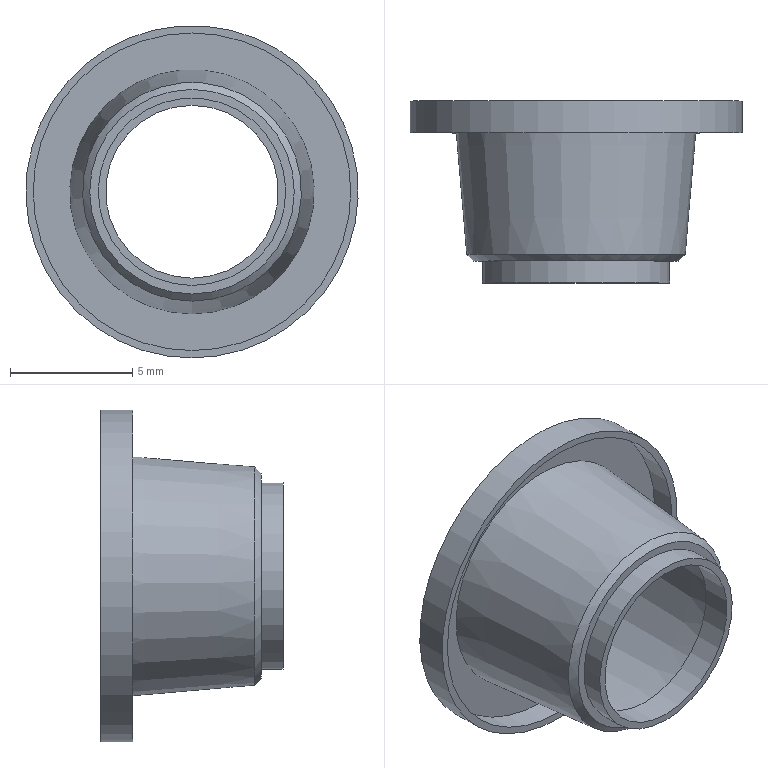Part | NX | features DATUM_CSYS 3, SKETCH 2, SWP104 1 | 1 solid | 13 faces | box 13.6 x 7.451 x 13.6 mm | volume 99.127 mm3 | plane 6 | cylinder 4 | cone 3 | commonest cylinder face diameters 7.073 x1 7.673 x1 13 x1 13.6 x1
STEP:
#1=CARTESIAN_POINT('',(0.,0.,-5.));
#2=VERTEX_POINT('',#1);
#3=CARTESIAN_POINT('',(0.,0.,0.));
#4=DIRECTION('',(0.,-1.,0.));
#5=DIRECTION('',(0.,0.,-1.));
#6=AXIS2_PLACEMENT_3D('',#3,#4,#5);
#7=CIRCLE('',#6,5.);
#8=EDGE_CURVE('',#2,#2,#7,.T.);
#9=ORIENTED_EDGE('',*,*,#8,.T.);
#10=EDGE_LOOP('',(#9));
#11=FACE_BOUND('',#10,.T.);
#12=CARTESIAN_POINT('',(0.,-5.977,-4.477));
#13=VERTEX_POINT('',#12);
#14=CARTESIAN_POINT('',(0.,-5.977,0.));
#15=DIRECTION('',(0.,-1.,0.));
#16=DIRECTION('',(0.,0.,-1.));
#17=AXIS2_PLACEMENT_3D('',#14,#15,#16);
#18=CIRCLE('',#17,4.477);
#19=EDGE_CURVE('',#13,#13,#18,.T.);
#20=ORIENTED_EDGE('',*,*,#19,.F.);
#21=EDGE_LOOP('',(#20));
#22=FACE_BOUND('',#21,.T.);
#23=CARTESIAN_POINT('',(0.,-5.977,0.));
#24=DIRECTION('',(0.,1.,0.));
#25=DIRECTION('',(0.,0.,1.));
#26=AXIS2_PLACEMENT_3D('',#23,#24,#25);
#27=CONICAL_SURFACE('',#26,4.477,0.08727);
#28=ADVANCED_FACE('',(#11,#22),#27,.T.);
#29=CARTESIAN_POINT('',(0.,0.,-6.5));
#30=VERTEX_POINT('',#29);
#31=CARTESIAN_POINT('',(0.,0.,0.));
#32=DIRECTION('',(0.,-1.,0.));
#33=DIRECTION('',(0.,0.,-1.));
#34=AXIS2_PLACEMENT_3D('',#31,#32,#33);
#35=CIRCLE('',#34,6.5);
#36=EDGE_CURVE('',#30,#30,#35,.T.);
#37=ORIENTED_EDGE('',*,*,#36,.T.);
#38=EDGE_LOOP('',(#37));
#39=FACE_BOUND('',#38,.T.);
#40=ORIENTED_EDGE('',*,*,#8,.F.);
#41=EDGE_LOOP('',(#40));
#42=FACE_BOUND('',#41,.T.);
#43=CARTESIAN_POINT('',(0.,0.,5.));
#44=DIRECTION('',(0.,-1.,0.));
#45=DIRECTION('',(0.,0.,-1.));
#46=AXIS2_PLACEMENT_3D('',#43,#44,#45);
#47=PLANE('',#46);
#48=ADVANCED_FACE('',(#39,#42),#47,.T.);
#49=CARTESIAN_POINT('',(0.,-1.,-6.5));
#50=VERTEX_POINT('',#49);
#51=CARTESIAN_POINT('',(0.,-1.,0.));
#52=DIRECTION('',(0.,-1.,0.));
#53=DIRECTION('',(0.,0.,-1.));
#54=AXIS2_PLACEMENT_3D('',#51,#52,#53);
#55=CIRCLE('',#54,6.5);
#56=EDGE_CURVE('',#50,#50,#55,.T.);
#57=ORIENTED_EDGE('',*,*,#56,.T.);
#58=EDGE_LOOP('',(#57));
#59=FACE_BOUND('',#58,.T.);
#60=ORIENTED_EDGE('',*,*,#36,.F.);
#61=EDGE_LOOP('',(#60));
#62=FACE_BOUND('',#61,.T.);
#63=CARTESIAN_POINT('',(0.,0.,0.));
#64=DIRECTION('',(0.,-1.,0.));
#65=DIRECTION('',(0.,0.,-1.));
#66=AXIS2_PLACEMENT_3D('',#63,#64,#65);
#67=CYLINDRICAL_SURFACE('',#66,6.5);
#68=ADVANCED_FACE('',(#59,#62),#67,.F.);
#69=CARTESIAN_POINT('',(0.,-1.,-6.8));
#70=VERTEX_POINT('',#69);
#71=CARTESIAN_POINT('',(0.,-1.,0.));
#72=DIRECTION('',(0.,-1.,0.));
#73=DIRECTION('',(0.,0.,-1.));
#74=AXIS2_PLACEMENT_3D('',#71,#72,#73);
#75=CIRCLE('',#74,6.8);
#76=EDGE_CURVE('',#70,#70,#75,.T.);
#77=ORIENTED_EDGE('',*,*,#76,.T.);
#78=EDGE_LOOP('',(#77));
#79=FACE_BOUND('',#78,.T.);
#80=ORIENTED_EDGE('',*,*,#56,.F.);
#81=EDGE_LOOP('',(#80));
#82=FACE_BOUND('',#81,.T.);
#83=CARTESIAN_POINT('',(0.,-1.,6.5));
#84=DIRECTION('',(0.,-1.,0.));
#85=DIRECTION('',(0.,0.,-1.));
#86=AXIS2_PLACEMENT_3D('',#83,#84,#85);
#87=PLANE('',#86);
#88=ADVANCED_FACE('',(#79,#82),#87,.T.);
#89=CARTESIAN_POINT('',(0.,0.3,-6.8));
#90=VERTEX_POINT('',#89);
#91=CARTESIAN_POINT('',(0.,0.3,0.));
#92=DIRECTION('',(0.,-1.,0.));
#93=DIRECTION('',(0.,0.,-1.));
#94=AXIS2_PLACEMENT_3D('',#91,#92,#93);
#95=CIRCLE('',#94,6.8);
#96=EDGE_CURVE('',#90,#90,#95,.T.);
#97=ORIENTED_EDGE('',*,*,#96,.T.);
#98=EDGE_LOOP('',(#97));
#99=FACE_BOUND('',#98,.T.);
#100=ORIENTED_EDGE('',*,*,#76,.F.);
#101=EDGE_LOOP('',(#100));
#102=FACE_BOUND('',#101,.T.);
#103=CARTESIAN_POINT('',(0.,0.,0.));
#104=DIRECTION('',(0.,-1.,0.));
#105=DIRECTION('',(0.,0.,-1.));
#106=AXIS2_PLACEMENT_3D('',#103,#104,#105);
#107=CYLINDRICAL_SURFACE('',#106,6.8);
#108=ADVANCED_FACE('',(#99,#102),#107,.T.);
#109=CARTESIAN_POINT('',(0.,0.3,-4.725));
#110=VERTEX_POINT('',#109);
#111=CARTESIAN_POINT('',(0.,0.3,0.));
#112=DIRECTION('',(0.,-1.,0.));
#113=DIRECTION('',(0.,0.,-1.));
#114=AXIS2_PLACEMENT_3D('',#111,#112,#113);
#115=CIRCLE('',#114,4.725);
#116=EDGE_CURVE('',#110,#110,#115,.T.);
#117=ORIENTED_EDGE('',*,*,#116,.T.);
#118=EDGE_LOOP('',(#117));
#119=FACE_BOUND('',#118,.T.);
#120=ORIENTED_EDGE('',*,*,#96,.F.);
#121=EDGE_LOOP('',(#120));
#122=FACE_BOUND('',#121,.T.);
#123=CARTESIAN_POINT('',(0.,0.3,6.8));
#124=DIRECTION('',(0.,1.,0.));
#125=DIRECTION('',(0.,0.,1.));
#126=AXIS2_PLACEMENT_3D('',#123,#124,#125);
#127=PLANE('',#126);
#128=ADVANCED_FACE('',(#119,#122),#127,.T.);
#129=CARTESIAN_POINT('',(0.,-5.951,-4.178));
#130=VERTEX_POINT('',#129);
#131=CARTESIAN_POINT('',(0.,-5.951,0.));
#132=DIRECTION('',(0.,-1.,0.));
#133=DIRECTION('',(0.,0.,-1.));
#134=AXIS2_PLACEMENT_3D('',#131,#132,#133);
#135=CIRCLE('',#134,4.178);
#136=EDGE_CURVE('',#130,#130,#135,.T.);
#137=ORIENTED_EDGE('',*,*,#136,.T.);
#138=EDGE_LOOP('',(#137));
#139=FACE_BOUND('',#138,.T.);
#140=ORIENTED_EDGE('',*,*,#116,.F.);
#141=EDGE_LOOP('',(#140));
#142=FACE_BOUND('',#141,.T.);
#143=CARTESIAN_POINT('',(0.,0.3,0.));
#144=DIRECTION('',(0.,1.,0.));
#145=DIRECTION('',(0.,0.,1.));
#146=AXIS2_PLACEMENT_3D('',#143,#144,#145);
#147=CONICAL_SURFACE('',#146,4.725,0.08727);
#148=ADVANCED_FACE('',(#139,#142),#147,.F.);
#149=CARTESIAN_POINT('',(0.,-5.951,-3.537));
#150=VERTEX_POINT('',#149);
#151=CARTESIAN_POINT('',(0.,-5.951,0.));
#152=DIRECTION('',(0.,-1.,0.));
#153=DIRECTION('',(0.,0.,-1.));
#154=AXIS2_PLACEMENT_3D('',#151,#152,#153);
#155=CIRCLE('',#154,3.537);
#156=EDGE_CURVE('',#150,#150,#155,.T.);
#157=ORIENTED_EDGE('',*,*,#156,.T.);
#158=EDGE_LOOP('',(#157));
#159=FACE_BOUND('',#158,.T.);
#160=ORIENTED_EDGE('',*,*,#136,.F.);
#161=EDGE_LOOP('',(#160));
#162=FACE_BOUND('',#161,.T.);
#163=CARTESIAN_POINT('',(0.,-5.951,4.178));
#164=DIRECTION('',(0.,1.,0.));
#165=DIRECTION('',(0.,0.,1.));
#166=AXIS2_PLACEMENT_3D('',#163,#164,#165);
#167=PLANE('',#166);
#168=ADVANCED_FACE('',(#159,#162),#167,.T.);
#169=CARTESIAN_POINT('',(0.,-7.151,-3.537));
#170=VERTEX_POINT('',#169);
#171=CARTESIAN_POINT('',(0.,-7.151,0.));
#172=DIRECTION('',(0.,-1.,0.));
#173=DIRECTION('',(0.,0.,-1.));
#174=AXIS2_PLACEMENT_3D('',#171,#172,#173);
#175=CIRCLE('',#174,3.537);
#176=EDGE_CURVE('',#170,#170,#175,.T.);
#177=ORIENTED_EDGE('',*,*,#176,.T.);
#178=EDGE_LOOP('',(#177));
#179=FACE_BOUND('',#178,.T.);
#180=ORIENTED_EDGE('',*,*,#156,.F.);
#181=EDGE_LOOP('',(#180));
#182=FACE_BOUND('',#181,.T.);
#183=CARTESIAN_POINT('',(0.,0.,0.));
#184=DIRECTION('',(0.,-1.,0.));
#185=DIRECTION('',(0.,0.,-1.));
#186=AXIS2_PLACEMENT_3D('',#183,#184,#185);
#187=CYLINDRICAL_SURFACE('',#186,3.537);
#188=ADVANCED_FACE('',(#179,#182),#187,.F.);
#189=CARTESIAN_POINT('',(0.,-7.151,-3.837));
#190=VERTEX_POINT('',#189);
#191=CARTESIAN_POINT('',(0.,-7.151,0.));
#192=DIRECTION('',(0.,-1.,0.));
#193=DIRECTION('',(0.,0.,-1.));
#194=AXIS2_PLACEMENT_3D('',#191,#192,#193);
#195=CIRCLE('',#194,3.837);
#196=EDGE_CURVE('',#190,#190,#195,.T.);
#197=ORIENTED_EDGE('',*,*,#196,.T.);
#198=EDGE_LOOP('',(#197));
#199=FACE_BOUND('',#198,.T.);
#200=ORIENTED_EDGE('',*,*,#176,.F.);
#201=EDGE_LOOP('',(#200));
#202=FACE_BOUND('',#201,.T.);
#203=CARTESIAN_POINT('',(0.,-7.151,3.537));
#204=DIRECTION('',(0.,-1.,0.));
#205=DIRECTION('',(0.,0.,-1.));
#206=AXIS2_PLACEMENT_3D('',#203,#204,#205);
#207=PLANE('',#206);
#208=ADVANCED_FACE('',(#199,#202),#207,.T.);
#209=CARTESIAN_POINT('',(0.,-6.251,-3.837));
#210=VERTEX_POINT('',#209);
#211=CARTESIAN_POINT('',(0.,-6.251,0.));
#212=DIRECTION('',(0.,-1.,0.));
#213=DIRECTION('',(0.,0.,-1.));
#214=AXIS2_PLACEMENT_3D('',#211,#212,#213);
#215=CIRCLE('',#214,3.837);
#216=EDGE_CURVE('',#210,#210,#215,.T.);
#217=ORIENTED_EDGE('',*,*,#216,.T.);
#218=EDGE_LOOP('',(#217));
#219=FACE_BOUND('',#218,.T.);
#220=ORIENTED_EDGE('',*,*,#196,.F.);
#221=EDGE_LOOP('',(#220));
#222=FACE_BOUND('',#221,.T.);
#223=CARTESIAN_POINT('',(0.,0.,0.));
#224=DIRECTION('',(0.,-1.,0.));
#225=DIRECTION('',(0.,0.,-1.));
#226=AXIS2_PLACEMENT_3D('',#223,#224,#225);
#227=CYLINDRICAL_SURFACE('',#226,3.837);
#228=ADVANCED_FACE('',(#219,#222),#227,.T.);
#229=CARTESIAN_POINT('',(0.,-6.251,-4.187));
#230=VERTEX_POINT('',#229);
#231=CARTESIAN_POINT('',(0.,-6.251,0.));
#232=DIRECTION('',(0.,-1.,0.));
#233=DIRECTION('',(0.,0.,-1.));
#234=AXIS2_PLACEMENT_3D('',#231,#232,#233);
#235=CIRCLE('',#234,4.187);
#236=EDGE_CURVE('',#230,#230,#235,.T.);
#237=ORIENTED_EDGE('',*,*,#236,.T.);
#238=EDGE_LOOP('',(#237));
#239=FACE_BOUND('',#238,.T.);
#240=ORIENTED_EDGE('',*,*,#216,.F.);
#241=EDGE_LOOP('',(#240));
#242=FACE_BOUND('',#241,.T.);
#243=CARTESIAN_POINT('',(0.,-6.251,3.837));
#244=DIRECTION('',(0.,-1.,0.));
#245=DIRECTION('',(0.,0.,-1.));
#246=AXIS2_PLACEMENT_3D('',#243,#244,#245);
#247=PLANE('',#246);
#248=ADVANCED_FACE('',(#239,#242),#247,.T.);
#249=ORIENTED_EDGE('',*,*,#19,.T.);
#250=EDGE_LOOP('',(#249));
#251=FACE_BOUND('',#250,.T.);
#252=ORIENTED_EDGE('',*,*,#236,.F.);
#253=EDGE_LOOP('',(#252));
#254=FACE_BOUND('',#253,.T.);
#255=CARTESIAN_POINT('',(0.,-6.251,0.));
#256=DIRECTION('',(0.,1.,0.));
#257=DIRECTION('',(0.,0.,1.));
#258=AXIS2_PLACEMENT_3D('',#255,#256,#257);
#259=CONICAL_SURFACE('',#258,4.187,0.8148);
#260=ADVANCED_FACE('',(#251,#254),#259,.T.);
#261=CLOSED_SHELL('',(#28,#48,#68,#88,#108,#128,#148,#168,#188,#208,#228,#248,#260));
#262=MANIFOLD_SOLID_BREP('',#261);
#263=(LENGTH_UNIT()NAMED_UNIT(*)SI_UNIT(.MILLI.,.METRE.));
#264=UNCERTAINTY_MEASURE_WITH_UNIT(LENGTH_MEASURE(0.00001),#263,'','');
#265=(NAMED_UNIT(*)PLANE_ANGLE_UNIT()SI_UNIT($,.RADIAN.));
#266=(NAMED_UNIT(*)SI_UNIT($,.STERADIAN.)SOLID_ANGLE_UNIT());
#267=(GEOMETRIC_REPRESENTATION_CONTEXT(3)GLOBAL_UNCERTAINTY_ASSIGNED_CONTEXT((#264))GLOBAL_UNIT_ASSIGNED_CONTEXT((#263,#265,#266))REPRESENTATION_CONTEXT('',''));
#268=ADVANCED_BREP_SHAPE_REPRESENTATION('',(#262),#267);